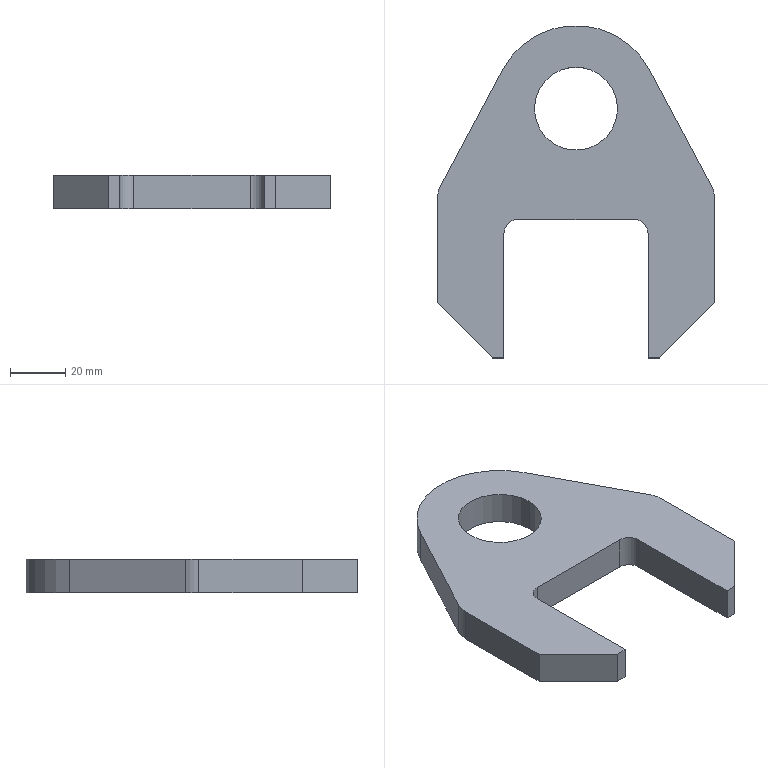Part | SolidWorks | features Extrusion 1 | 1 solid | 20 faces | box 100 x 120 x 12 mm | volume 75307 mm3 | plane 13 | cylinder 7 | commonest cylinder face diameters 10 x2 20 x2 30 x2 60 x1
STEP:
#1=CARTESIAN_POINT('',(-15.,90.,6.));
#2=VERTEX_POINT('',#1);
#3=CARTESIAN_POINT('',(15.,90.,6.));
#4=VERTEX_POINT('',#3);
#5=CARTESIAN_POINT('',(0.,90.,6.));
#6=DIRECTION('',(0.,0.,1.));
#7=DIRECTION('',(1.,0.,0.));
#8=AXIS2_PLACEMENT_3D('',#5,#6,#7);
#9=CIRCLE('',#8,15.);
#10=EDGE_CURVE('',#2,#4,#9,.T.);
#11=ORIENTED_EDGE('',*,*,#10,.T.);
#12=CARTESIAN_POINT('',(15.,90.,-6.));
#13=VERTEX_POINT('',#12);
#14=CARTESIAN_POINT('',(15.,90.,6.));
#15=DIRECTION('',(0.,0.,-1.));
#16=VECTOR('',#15,1000.);
#17=LINE('',#14,#16);
#18=EDGE_CURVE('',#4,#13,#17,.T.);
#19=ORIENTED_EDGE('',*,*,#18,.T.);
#20=CARTESIAN_POINT('',(-15.,90.,-6.));
#21=VERTEX_POINT('',#20);
#22=CARTESIAN_POINT('',(0.,90.,-6.));
#23=DIRECTION('',(0.,0.,1.));
#24=DIRECTION('',(1.,0.,0.));
#25=AXIS2_PLACEMENT_3D('',#22,#23,#24);
#26=CIRCLE('',#25,15.);
#27=EDGE_CURVE('',#21,#13,#26,.T.);
#28=ORIENTED_EDGE('',*,*,#27,.F.);
#29=CARTESIAN_POINT('',(-15.,90.,6.));
#30=DIRECTION('',(0.,0.,-1.));
#31=VECTOR('',#30,1000.);
#32=LINE('',#29,#31);
#33=EDGE_CURVE('',#2,#21,#32,.T.);
#34=ORIENTED_EDGE('',*,*,#33,.F.);
#35=EDGE_LOOP('',(#11,#19,#28,#34));
#36=FACE_OUTER_BOUND('',#35,.T.);
#37=CARTESIAN_POINT('',(0.,90.,6.));
#38=DIRECTION('',(0.,0.,-1.));
#39=DIRECTION('',(-1.,0.,0.));
#40=AXIS2_PLACEMENT_3D('',#37,#38,#39);
#41=CYLINDRICAL_SURFACE('',#40,15.);
#42=ADVANCED_FACE('',(#36),#41,.F.);
#43=CARTESIAN_POINT('',(-26.,0.,6.));
#44=VERTEX_POINT('',#43);
#45=CARTESIAN_POINT('',(-26.,45.,6.));
#46=VERTEX_POINT('',#45);
#47=CARTESIAN_POINT('',(-26.,0.,6.));
#48=DIRECTION('',(0.,1.,0.));
#49=VECTOR('',#48,1000.);
#50=LINE('',#47,#49);
#51=EDGE_CURVE('',#44,#46,#50,.T.);
#52=ORIENTED_EDGE('',*,*,#51,.T.);
#53=CARTESIAN_POINT('',(-21.,50.,6.));
#54=VERTEX_POINT('',#53);
#55=CARTESIAN_POINT('',(-21.,45.,6.));
#56=DIRECTION('',(0.,0.,-1.));
#57=DIRECTION('',(-1.,0.,0.));
#58=AXIS2_PLACEMENT_3D('',#55,#56,#57);
#59=CIRCLE('',#58,5.);
#60=EDGE_CURVE('',#46,#54,#59,.T.);
#61=ORIENTED_EDGE('',*,*,#60,.T.);
#62=CARTESIAN_POINT('',(21.,50.,6.));
#63=VERTEX_POINT('',#62);
#64=CARTESIAN_POINT('',(-21.,50.,6.));
#65=DIRECTION('',(1.,0.,0.));
#66=VECTOR('',#65,1000.);
#67=LINE('',#64,#66);
#68=EDGE_CURVE('',#54,#63,#67,.T.);
#69=ORIENTED_EDGE('',*,*,#68,.T.);
#70=CARTESIAN_POINT('',(26.,45.,6.));
#71=VERTEX_POINT('',#70);
#72=CARTESIAN_POINT('',(21.,45.,6.));
#73=DIRECTION('',(0.,0.,-1.));
#74=DIRECTION('',(1.,0.,0.));
#75=AXIS2_PLACEMENT_3D('',#72,#73,#74);
#76=CIRCLE('',#75,5.);
#77=EDGE_CURVE('',#63,#71,#76,.T.);
#78=ORIENTED_EDGE('',*,*,#77,.T.);
#79=CARTESIAN_POINT('',(26.,0.,6.));
#80=VERTEX_POINT('',#79);
#81=CARTESIAN_POINT('',(26.,0.,6.));
#82=DIRECTION('',(0.,-1.,0.));
#83=VECTOR('',#82,1000.);
#84=LINE('',#81,#83);
#85=EDGE_CURVE('',#71,#80,#84,.T.);
#86=ORIENTED_EDGE('',*,*,#85,.T.);
#87=CARTESIAN_POINT('',(30.,0.,6.));
#88=VERTEX_POINT('',#87);
#89=CARTESIAN_POINT('',(26.,0.,6.));
#90=DIRECTION('',(1.,0.,0.));
#91=VECTOR('',#90,1000.);
#92=LINE('',#89,#91);
#93=EDGE_CURVE('',#80,#88,#92,.T.);
#94=ORIENTED_EDGE('',*,*,#93,.T.);
#95=CARTESIAN_POINT('',(50.,20.,6.));
#96=VERTEX_POINT('',#95);
#97=CARTESIAN_POINT('',(30.,0.,6.));
#98=DIRECTION('',(0.7071,0.7071,0.));
#99=VECTOR('',#98,1000.);
#100=LINE('',#97,#99);
#101=EDGE_CURVE('',#88,#96,#100,.T.);
#102=ORIENTED_EDGE('',*,*,#101,.T.);
#103=CARTESIAN_POINT('',(50.,57.5,6.));
#104=VERTEX_POINT('',#103);
#105=CARTESIAN_POINT('',(50.,20.,6.));
#106=DIRECTION('',(0.,1.,0.));
#107=VECTOR('',#106,1000.);
#108=LINE('',#105,#107);
#109=EDGE_CURVE('',#96,#104,#108,.T.);
#110=ORIENTED_EDGE('',*,*,#109,.T.);
#111=CARTESIAN_POINT('',(48.824,62.206,6.));
#112=VERTEX_POINT('',#111);
#113=CARTESIAN_POINT('',(40.,57.5,6.));
#114=DIRECTION('',(0.,0.,1.));
#115=DIRECTION('',(-1.,0.,0.));
#116=AXIS2_PLACEMENT_3D('',#113,#114,#115);
#117=CIRCLE('',#116,10.);
#118=EDGE_CURVE('',#104,#112,#117,.T.);
#119=ORIENTED_EDGE('',*,*,#118,.T.);
#120=CARTESIAN_POINT('',(26.471,104.118,6.));
#121=VERTEX_POINT('',#120);
#122=CARTESIAN_POINT('',(48.824,62.206,6.));
#123=DIRECTION('',(-0.4706,0.8824,0.));
#124=VECTOR('',#123,1000.);
#125=LINE('',#122,#124);
#126=EDGE_CURVE('',#112,#121,#125,.T.);
#127=ORIENTED_EDGE('',*,*,#126,.T.);
#128=CARTESIAN_POINT('',(-26.471,104.118,6.));
#129=VERTEX_POINT('',#128);
#130=CARTESIAN_POINT('',(0.,90.,6.));
#131=DIRECTION('',(0.,0.,1.));
#132=DIRECTION('',(-1.,0.,0.));
#133=AXIS2_PLACEMENT_3D('',#130,#131,#132);
#134=CIRCLE('',#133,30.);
#135=EDGE_CURVE('',#121,#129,#134,.T.);
#136=ORIENTED_EDGE('',*,*,#135,.T.);
#137=CARTESIAN_POINT('',(-48.824,62.206,6.));
#138=VERTEX_POINT('',#137);
#139=CARTESIAN_POINT('',(-48.824,62.206,6.));
#140=DIRECTION('',(-0.4706,-0.8824,0.));
#141=VECTOR('',#140,1000.);
#142=LINE('',#139,#141);
#143=EDGE_CURVE('',#129,#138,#142,.T.);
#144=ORIENTED_EDGE('',*,*,#143,.T.);
#145=CARTESIAN_POINT('',(-50.,57.5,6.));
#146=VERTEX_POINT('',#145);
#147=CARTESIAN_POINT('',(-40.,57.5,6.));
#148=DIRECTION('',(0.,0.,1.));
#149=DIRECTION('',(-1.,0.,0.));
#150=AXIS2_PLACEMENT_3D('',#147,#148,#149);
#151=CIRCLE('',#150,10.);
#152=EDGE_CURVE('',#138,#146,#151,.T.);
#153=ORIENTED_EDGE('',*,*,#152,.T.);
#154=CARTESIAN_POINT('',(-50.,20.,6.));
#155=VERTEX_POINT('',#154);
#156=CARTESIAN_POINT('',(-50.,20.,6.));
#157=DIRECTION('',(0.,-1.,0.));
#158=VECTOR('',#157,1000.);
#159=LINE('',#156,#158);
#160=EDGE_CURVE('',#146,#155,#159,.T.);
#161=ORIENTED_EDGE('',*,*,#160,.T.);
#162=CARTESIAN_POINT('',(-30.,0.,6.));
#163=VERTEX_POINT('',#162);
#164=CARTESIAN_POINT('',(-30.,0.,6.));
#165=DIRECTION('',(0.7071,-0.7071,0.));
#166=VECTOR('',#165,1000.);
#167=LINE('',#164,#166);
#168=EDGE_CURVE('',#155,#163,#167,.T.);
#169=ORIENTED_EDGE('',*,*,#168,.T.);
#170=CARTESIAN_POINT('',(-26.,0.,6.));
#171=DIRECTION('',(1.,0.,0.));
#172=VECTOR('',#171,1000.);
#173=LINE('',#170,#172);
#174=EDGE_CURVE('',#163,#44,#173,.T.);
#175=ORIENTED_EDGE('',*,*,#174,.T.);
#176=EDGE_LOOP('',(#52,#61,#69,#78,#86,#94,#102,#110,#119,#127,#136,#144,#153,#161,#169,#175));
#177=FACE_OUTER_BOUND('',#176,.T.);
#178=ORIENTED_EDGE('',*,*,#10,.F.);
#179=CARTESIAN_POINT('',(0.,90.,6.));
#180=DIRECTION('',(0.,0.,1.));
#181=DIRECTION('',(1.,0.,0.));
#182=AXIS2_PLACEMENT_3D('',#179,#180,#181);
#183=CIRCLE('',#182,15.);
#184=EDGE_CURVE('',#4,#2,#183,.T.);
#185=ORIENTED_EDGE('',*,*,#184,.F.);
#186=EDGE_LOOP('',(#178,#185));
#187=FACE_BOUND('',#186,.T.);
#188=CARTESIAN_POINT('',(-21.,45.,6.));
#189=DIRECTION('',(0.,0.,-1.));
#190=DIRECTION('',(-1.,0.,0.));
#191=AXIS2_PLACEMENT_3D('',#188,#189,#190);
#192=PLANE('',#191);
#193=ADVANCED_FACE('',(#177,#187),#192,.F.);
#194=CARTESIAN_POINT('',(-26.,0.,-6.));
#195=VERTEX_POINT('',#194);
#196=CARTESIAN_POINT('',(-26.,45.,-6.));
#197=VERTEX_POINT('',#196);
#198=CARTESIAN_POINT('',(-26.,0.,-6.));
#199=DIRECTION('',(0.,1.,0.));
#200=VECTOR('',#199,1000.);
#201=LINE('',#198,#200);
#202=EDGE_CURVE('',#195,#197,#201,.T.);
#203=ORIENTED_EDGE('',*,*,#202,.F.);
#204=CARTESIAN_POINT('',(-30.,0.,-6.));
#205=VERTEX_POINT('',#204);
#206=CARTESIAN_POINT('',(-26.,0.,-6.));
#207=DIRECTION('',(1.,0.,0.));
#208=VECTOR('',#207,1000.);
#209=LINE('',#206,#208);
#210=EDGE_CURVE('',#205,#195,#209,.T.);
#211=ORIENTED_EDGE('',*,*,#210,.F.);
#212=CARTESIAN_POINT('',(-50.,20.,-6.));
#213=VERTEX_POINT('',#212);
#214=CARTESIAN_POINT('',(-30.,0.,-6.));
#215=DIRECTION('',(0.7071,-0.7071,0.));
#216=VECTOR('',#215,1000.);
#217=LINE('',#214,#216);
#218=EDGE_CURVE('',#213,#205,#217,.T.);
#219=ORIENTED_EDGE('',*,*,#218,.F.);
#220=CARTESIAN_POINT('',(-50.,57.5,-6.));
#221=VERTEX_POINT('',#220);
#222=CARTESIAN_POINT('',(-50.,20.,-6.));
#223=DIRECTION('',(0.,-1.,0.));
#224=VECTOR('',#223,1000.);
#225=LINE('',#222,#224);
#226=EDGE_CURVE('',#221,#213,#225,.T.);
#227=ORIENTED_EDGE('',*,*,#226,.F.);
#228=CARTESIAN_POINT('',(-48.824,62.206,-6.));
#229=VERTEX_POINT('',#228);
#230=CARTESIAN_POINT('',(-40.,57.5,-6.));
#231=DIRECTION('',(0.,0.,1.));
#232=DIRECTION('',(-1.,0.,0.));
#233=AXIS2_PLACEMENT_3D('',#230,#231,#232);
#234=CIRCLE('',#233,10.);
#235=EDGE_CURVE('',#229,#221,#234,.T.);
#236=ORIENTED_EDGE('',*,*,#235,.F.);
#237=CARTESIAN_POINT('',(-26.471,104.118,-6.));
#238=VERTEX_POINT('',#237);
#239=CARTESIAN_POINT('',(-48.824,62.206,-6.));
#240=DIRECTION('',(-0.4706,-0.8824,0.));
#241=VECTOR('',#240,1000.);
#242=LINE('',#239,#241);
#243=EDGE_CURVE('',#238,#229,#242,.T.);
#244=ORIENTED_EDGE('',*,*,#243,.F.);
#245=CARTESIAN_POINT('',(26.471,104.118,-6.));
#246=VERTEX_POINT('',#245);
#247=CARTESIAN_POINT('',(0.,90.,-6.));
#248=DIRECTION('',(0.,0.,1.));
#249=DIRECTION('',(-1.,0.,0.));
#250=AXIS2_PLACEMENT_3D('',#247,#248,#249);
#251=CIRCLE('',#250,30.);
#252=EDGE_CURVE('',#246,#238,#251,.T.);
#253=ORIENTED_EDGE('',*,*,#252,.F.);
#254=CARTESIAN_POINT('',(48.824,62.206,-6.));
#255=VERTEX_POINT('',#254);
#256=CARTESIAN_POINT('',(48.824,62.206,-6.));
#257=DIRECTION('',(-0.4706,0.8824,0.));
#258=VECTOR('',#257,1000.);
#259=LINE('',#256,#258);
#260=EDGE_CURVE('',#255,#246,#259,.T.);
#261=ORIENTED_EDGE('',*,*,#260,.F.);
#262=CARTESIAN_POINT('',(50.,57.5,-6.));
#263=VERTEX_POINT('',#262);
#264=CARTESIAN_POINT('',(40.,57.5,-6.));
#265=DIRECTION('',(0.,0.,1.));
#266=DIRECTION('',(-1.,0.,0.));
#267=AXIS2_PLACEMENT_3D('',#264,#265,#266);
#268=CIRCLE('',#267,10.);
#269=EDGE_CURVE('',#263,#255,#268,.T.);
#270=ORIENTED_EDGE('',*,*,#269,.F.);
#271=CARTESIAN_POINT('',(50.,20.,-6.));
#272=VERTEX_POINT('',#271);
#273=CARTESIAN_POINT('',(50.,20.,-6.));
#274=DIRECTION('',(0.,1.,0.));
#275=VECTOR('',#274,1000.);
#276=LINE('',#273,#275);
#277=EDGE_CURVE('',#272,#263,#276,.T.);
#278=ORIENTED_EDGE('',*,*,#277,.F.);
#279=CARTESIAN_POINT('',(30.,0.,-6.));
#280=VERTEX_POINT('',#279);
#281=CARTESIAN_POINT('',(30.,0.,-6.));
#282=DIRECTION('',(0.7071,0.7071,0.));
#283=VECTOR('',#282,1000.);
#284=LINE('',#281,#283);
#285=EDGE_CURVE('',#280,#272,#284,.T.);
#286=ORIENTED_EDGE('',*,*,#285,.F.);
#287=CARTESIAN_POINT('',(26.,0.,-6.));
#288=VERTEX_POINT('',#287);
#289=CARTESIAN_POINT('',(26.,0.,-6.));
#290=DIRECTION('',(1.,0.,0.));
#291=VECTOR('',#290,1000.);
#292=LINE('',#289,#291);
#293=EDGE_CURVE('',#288,#280,#292,.T.);
#294=ORIENTED_EDGE('',*,*,#293,.F.);
#295=CARTESIAN_POINT('',(26.,45.,-6.));
#296=VERTEX_POINT('',#295);
#297=CARTESIAN_POINT('',(26.,0.,-6.));
#298=DIRECTION('',(0.,-1.,0.));
#299=VECTOR('',#298,1000.);
#300=LINE('',#297,#299);
#301=EDGE_CURVE('',#296,#288,#300,.T.);
#302=ORIENTED_EDGE('',*,*,#301,.F.);
#303=CARTESIAN_POINT('',(21.,50.,-6.));
#304=VERTEX_POINT('',#303);
#305=CARTESIAN_POINT('',(21.,45.,-6.));
#306=DIRECTION('',(0.,0.,-1.));
#307=DIRECTION('',(1.,0.,0.));
#308=AXIS2_PLACEMENT_3D('',#305,#306,#307);
#309=CIRCLE('',#308,5.);
#310=EDGE_CURVE('',#304,#296,#309,.T.);
#311=ORIENTED_EDGE('',*,*,#310,.F.);
#312=CARTESIAN_POINT('',(-21.,50.,-6.));
#313=VERTEX_POINT('',#312);
#314=CARTESIAN_POINT('',(-21.,50.,-6.));
#315=DIRECTION('',(1.,0.,0.));
#316=VECTOR('',#315,1000.);
#317=LINE('',#314,#316);
#318=EDGE_CURVE('',#313,#304,#317,.T.);
#319=ORIENTED_EDGE('',*,*,#318,.F.);
#320=CARTESIAN_POINT('',(-21.,45.,-6.));
#321=DIRECTION('',(0.,0.,-1.));
#322=DIRECTION('',(-1.,0.,0.));
#323=AXIS2_PLACEMENT_3D('',#320,#321,#322);
#324=CIRCLE('',#323,5.);
#325=EDGE_CURVE('',#197,#313,#324,.T.);
#326=ORIENTED_EDGE('',*,*,#325,.F.);
#327=EDGE_LOOP('',(#203,#211,#219,#227,#236,#244,#253,#261,#270,#278,#286,#294,#302,#311,#319,#326));
#328=FACE_OUTER_BOUND('',#327,.T.);
#329=ORIENTED_EDGE('',*,*,#27,.T.);
#330=CARTESIAN_POINT('',(0.,90.,-6.));
#331=DIRECTION('',(0.,0.,1.));
#332=DIRECTION('',(1.,0.,0.));
#333=AXIS2_PLACEMENT_3D('',#330,#331,#332);
#334=CIRCLE('',#333,15.);
#335=EDGE_CURVE('',#13,#21,#334,.T.);
#336=ORIENTED_EDGE('',*,*,#335,.T.);
#337=EDGE_LOOP('',(#329,#336));
#338=FACE_BOUND('',#337,.T.);
#339=CARTESIAN_POINT('',(-21.,45.,-6.));
#340=DIRECTION('',(0.,0.,-1.));
#341=DIRECTION('',(-1.,0.,0.));
#342=AXIS2_PLACEMENT_3D('',#339,#340,#341);
#343=PLANE('',#342);
#344=ADVANCED_FACE('',(#328,#338),#343,.T.);
#345=ORIENTED_EDGE('',*,*,#202,.T.);
#346=CARTESIAN_POINT('',(-26.,45.,6.));
#347=DIRECTION('',(0.,0.,-1.));
#348=VECTOR('',#347,1000.);
#349=LINE('',#346,#348);
#350=EDGE_CURVE('',#46,#197,#349,.T.);
#351=ORIENTED_EDGE('',*,*,#350,.F.);
#352=ORIENTED_EDGE('',*,*,#51,.F.);
#353=CARTESIAN_POINT('',(-26.,0.,6.));
#354=DIRECTION('',(0.,0.,-1.));
#355=VECTOR('',#354,1000.);
#356=LINE('',#353,#355);
#357=EDGE_CURVE('',#44,#195,#356,.T.);
#358=ORIENTED_EDGE('',*,*,#357,.T.);
#359=EDGE_LOOP('',(#345,#351,#352,#358));
#360=FACE_OUTER_BOUND('',#359,.T.);
#361=CARTESIAN_POINT('',(-26.,0.,6.));
#362=DIRECTION('',(-1.,0.,0.));
#363=DIRECTION('',(0.,0.,1.));
#364=AXIS2_PLACEMENT_3D('',#361,#362,#363);
#365=PLANE('',#364);
#366=ADVANCED_FACE('',(#360),#365,.F.);
#367=ORIENTED_EDGE('',*,*,#325,.T.);
#368=CARTESIAN_POINT('',(-21.,50.,6.));
#369=DIRECTION('',(0.,0.,-1.));
#370=VECTOR('',#369,1000.);
#371=LINE('',#368,#370);
#372=EDGE_CURVE('',#54,#313,#371,.T.);
#373=ORIENTED_EDGE('',*,*,#372,.F.);
#374=ORIENTED_EDGE('',*,*,#60,.F.);
#375=ORIENTED_EDGE('',*,*,#350,.T.);
#376=EDGE_LOOP('',(#367,#373,#374,#375));
#377=FACE_OUTER_BOUND('',#376,.T.);
#378=CARTESIAN_POINT('',(-21.,45.,6.));
#379=DIRECTION('',(0.,0.,-1.));
#380=DIRECTION('',(-1.,0.,0.));
#381=AXIS2_PLACEMENT_3D('',#378,#379,#380);
#382=CYLINDRICAL_SURFACE('',#381,5.);
#383=ADVANCED_FACE('',(#377),#382,.F.);
#384=ORIENTED_EDGE('',*,*,#318,.T.);
#385=CARTESIAN_POINT('',(21.,50.,6.));
#386=DIRECTION('',(0.,0.,-1.));
#387=VECTOR('',#386,1000.);
#388=LINE('',#385,#387);
#389=EDGE_CURVE('',#63,#304,#388,.T.);
#390=ORIENTED_EDGE('',*,*,#389,.F.);
#391=ORIENTED_EDGE('',*,*,#68,.F.);
#392=ORIENTED_EDGE('',*,*,#372,.T.);
#393=EDGE_LOOP('',(#384,#390,#391,#392));
#394=FACE_OUTER_BOUND('',#393,.T.);
#395=CARTESIAN_POINT('',(-21.,50.,6.));
#396=DIRECTION('',(0.,1.,0.));
#397=DIRECTION('',(0.,0.,1.));
#398=AXIS2_PLACEMENT_3D('',#395,#396,#397);
#399=PLANE('',#398);
#400=ADVANCED_FACE('',(#394),#399,.F.);
#401=ORIENTED_EDGE('',*,*,#310,.T.);
#402=CARTESIAN_POINT('',(26.,45.,6.));
#403=DIRECTION('',(0.,0.,-1.));
#404=VECTOR('',#403,1000.);
#405=LINE('',#402,#404);
#406=EDGE_CURVE('',#71,#296,#405,.T.);
#407=ORIENTED_EDGE('',*,*,#406,.F.);
#408=ORIENTED_EDGE('',*,*,#77,.F.);
#409=ORIENTED_EDGE('',*,*,#389,.T.);
#410=EDGE_LOOP('',(#401,#407,#408,#409));
#411=FACE_OUTER_BOUND('',#410,.T.);
#412=CARTESIAN_POINT('',(21.,45.,6.));
#413=DIRECTION('',(0.,0.,-1.));
#414=DIRECTION('',(-1.,0.,0.));
#415=AXIS2_PLACEMENT_3D('',#412,#413,#414);
#416=CYLINDRICAL_SURFACE('',#415,5.);
#417=ADVANCED_FACE('',(#411),#416,.F.);
#418=ORIENTED_EDGE('',*,*,#301,.T.);
#419=CARTESIAN_POINT('',(26.,0.,6.));
#420=DIRECTION('',(0.,0.,-1.));
#421=VECTOR('',#420,1000.);
#422=LINE('',#419,#421);
#423=EDGE_CURVE('',#80,#288,#422,.T.);
#424=ORIENTED_EDGE('',*,*,#423,.F.);
#425=ORIENTED_EDGE('',*,*,#85,.F.);
#426=ORIENTED_EDGE('',*,*,#406,.T.);
#427=EDGE_LOOP('',(#418,#424,#425,#426));
#428=FACE_OUTER_BOUND('',#427,.T.);
#429=CARTESIAN_POINT('',(26.,0.,6.));
#430=DIRECTION('',(1.,0.,0.));
#431=DIRECTION('',(0.,0.,-1.));
#432=AXIS2_PLACEMENT_3D('',#429,#430,#431);
#433=PLANE('',#432);
#434=ADVANCED_FACE('',(#428),#433,.F.);
#435=ORIENTED_EDGE('',*,*,#293,.T.);
#436=CARTESIAN_POINT('',(30.,0.,6.));
#437=DIRECTION('',(0.,0.,-1.));
#438=VECTOR('',#437,1000.);
#439=LINE('',#436,#438);
#440=EDGE_CURVE('',#88,#280,#439,.T.);
#441=ORIENTED_EDGE('',*,*,#440,.F.);
#442=ORIENTED_EDGE('',*,*,#93,.F.);
#443=ORIENTED_EDGE('',*,*,#423,.T.);
#444=EDGE_LOOP('',(#435,#441,#442,#443));
#445=FACE_OUTER_BOUND('',#444,.T.);
#446=CARTESIAN_POINT('',(26.,0.,6.));
#447=DIRECTION('',(0.,1.,0.));
#448=DIRECTION('',(-1.,0.,0.));
#449=AXIS2_PLACEMENT_3D('',#446,#447,#448);
#450=PLANE('',#449);
#451=ADVANCED_FACE('',(#445),#450,.F.);
#452=ORIENTED_EDGE('',*,*,#285,.T.);
#453=CARTESIAN_POINT('',(50.,20.,6.));
#454=DIRECTION('',(0.,0.,-1.));
#455=VECTOR('',#454,1000.);
#456=LINE('',#453,#455);
#457=EDGE_CURVE('',#96,#272,#456,.T.);
#458=ORIENTED_EDGE('',*,*,#457,.F.);
#459=ORIENTED_EDGE('',*,*,#101,.F.);
#460=ORIENTED_EDGE('',*,*,#440,.T.);
#461=EDGE_LOOP('',(#452,#458,#459,#460));
#462=FACE_OUTER_BOUND('',#461,.T.);
#463=CARTESIAN_POINT('',(30.,0.,6.));
#464=DIRECTION('',(-0.7071,0.7071,0.));
#465=DIRECTION('',(-0.7071,-0.7071,0.));
#466=AXIS2_PLACEMENT_3D('',#463,#464,#465);
#467=PLANE('',#466);
#468=ADVANCED_FACE('',(#462),#467,.F.);
#469=ORIENTED_EDGE('',*,*,#277,.T.);
#470=CARTESIAN_POINT('',(50.,57.5,6.));
#471=DIRECTION('',(0.,0.,-1.));
#472=VECTOR('',#471,1000.);
#473=LINE('',#470,#472);
#474=EDGE_CURVE('',#104,#263,#473,.T.);
#475=ORIENTED_EDGE('',*,*,#474,.F.);
#476=ORIENTED_EDGE('',*,*,#109,.F.);
#477=ORIENTED_EDGE('',*,*,#457,.T.);
#478=EDGE_LOOP('',(#469,#475,#476,#477));
#479=FACE_OUTER_BOUND('',#478,.T.);
#480=CARTESIAN_POINT('',(50.,20.,6.));
#481=DIRECTION('',(-1.,0.,0.));
#482=DIRECTION('',(0.,0.,1.));
#483=AXIS2_PLACEMENT_3D('',#480,#481,#482);
#484=PLANE('',#483);
#485=ADVANCED_FACE('',(#479),#484,.F.);
#486=ORIENTED_EDGE('',*,*,#269,.T.);
#487=CARTESIAN_POINT('',(48.824,62.206,6.));
#488=DIRECTION('',(0.,0.,-1.));
#489=VECTOR('',#488,1000.);
#490=LINE('',#487,#489);
#491=EDGE_CURVE('',#112,#255,#490,.T.);
#492=ORIENTED_EDGE('',*,*,#491,.F.);
#493=ORIENTED_EDGE('',*,*,#118,.F.);
#494=ORIENTED_EDGE('',*,*,#474,.T.);
#495=EDGE_LOOP('',(#486,#492,#493,#494));
#496=FACE_OUTER_BOUND('',#495,.T.);
#497=CARTESIAN_POINT('',(40.,57.5,6.));
#498=DIRECTION('',(0.,0.,-1.));
#499=DIRECTION('',(-1.,0.,0.));
#500=AXIS2_PLACEMENT_3D('',#497,#498,#499);
#501=CYLINDRICAL_SURFACE('',#500,10.);
#502=ADVANCED_FACE('',(#496),#501,.T.);
#503=ORIENTED_EDGE('',*,*,#260,.T.);
#504=CARTESIAN_POINT('',(26.471,104.118,6.));
#505=DIRECTION('',(0.,0.,-1.));
#506=VECTOR('',#505,1000.);
#507=LINE('',#504,#506);
#508=EDGE_CURVE('',#121,#246,#507,.T.);
#509=ORIENTED_EDGE('',*,*,#508,.F.);
#510=ORIENTED_EDGE('',*,*,#126,.F.);
#511=ORIENTED_EDGE('',*,*,#491,.T.);
#512=EDGE_LOOP('',(#503,#509,#510,#511));
#513=FACE_OUTER_BOUND('',#512,.T.);
#514=CARTESIAN_POINT('',(48.824,62.206,6.));
#515=DIRECTION('',(-0.8824,-0.4706,0.));
#516=DIRECTION('',(0.4706,-0.8824,0.));
#517=AXIS2_PLACEMENT_3D('',#514,#515,#516);
#518=PLANE('',#517);
#519=ADVANCED_FACE('',(#513),#518,.F.);
#520=ORIENTED_EDGE('',*,*,#252,.T.);
#521=CARTESIAN_POINT('',(-26.471,104.118,6.));
#522=DIRECTION('',(0.,0.,-1.));
#523=VECTOR('',#522,1000.);
#524=LINE('',#521,#523);
#525=EDGE_CURVE('',#129,#238,#524,.T.);
#526=ORIENTED_EDGE('',*,*,#525,.F.);
#527=ORIENTED_EDGE('',*,*,#135,.F.);
#528=ORIENTED_EDGE('',*,*,#508,.T.);
#529=EDGE_LOOP('',(#520,#526,#527,#528));
#530=FACE_OUTER_BOUND('',#529,.T.);
#531=CARTESIAN_POINT('',(0.,90.,6.));
#532=DIRECTION('',(0.,0.,-1.));
#533=DIRECTION('',(-1.,0.,0.));
#534=AXIS2_PLACEMENT_3D('',#531,#532,#533);
#535=CYLINDRICAL_SURFACE('',#534,30.);
#536=ADVANCED_FACE('',(#530),#535,.T.);
#537=ORIENTED_EDGE('',*,*,#243,.T.);
#538=CARTESIAN_POINT('',(-48.824,62.206,6.));
#539=DIRECTION('',(0.,0.,-1.));
#540=VECTOR('',#539,1000.);
#541=LINE('',#538,#540);
#542=EDGE_CURVE('',#138,#229,#541,.T.);
#543=ORIENTED_EDGE('',*,*,#542,.F.);
#544=ORIENTED_EDGE('',*,*,#143,.F.);
#545=ORIENTED_EDGE('',*,*,#525,.T.);
#546=EDGE_LOOP('',(#537,#543,#544,#545));
#547=FACE_OUTER_BOUND('',#546,.T.);
#548=CARTESIAN_POINT('',(-48.824,62.206,6.));
#549=DIRECTION('',(0.8824,-0.4706,0.));
#550=DIRECTION('',(0.4706,0.8824,0.));
#551=AXIS2_PLACEMENT_3D('',#548,#549,#550);
#552=PLANE('',#551);
#553=ADVANCED_FACE('',(#547),#552,.F.);
#554=ORIENTED_EDGE('',*,*,#235,.T.);
#555=CARTESIAN_POINT('',(-50.,57.5,6.));
#556=DIRECTION('',(0.,0.,-1.));
#557=VECTOR('',#556,1000.);
#558=LINE('',#555,#557);
#559=EDGE_CURVE('',#146,#221,#558,.T.);
#560=ORIENTED_EDGE('',*,*,#559,.F.);
#561=ORIENTED_EDGE('',*,*,#152,.F.);
#562=ORIENTED_EDGE('',*,*,#542,.T.);
#563=EDGE_LOOP('',(#554,#560,#561,#562));
#564=FACE_OUTER_BOUND('',#563,.T.);
#565=CARTESIAN_POINT('',(-40.,57.5,6.));
#566=DIRECTION('',(0.,0.,-1.));
#567=DIRECTION('',(-1.,0.,0.));
#568=AXIS2_PLACEMENT_3D('',#565,#566,#567);
#569=CYLINDRICAL_SURFACE('',#568,10.);
#570=ADVANCED_FACE('',(#564),#569,.T.);
#571=ORIENTED_EDGE('',*,*,#226,.T.);
#572=CARTESIAN_POINT('',(-50.,20.,6.));
#573=DIRECTION('',(0.,0.,-1.));
#574=VECTOR('',#573,1000.);
#575=LINE('',#572,#574);
#576=EDGE_CURVE('',#155,#213,#575,.T.);
#577=ORIENTED_EDGE('',*,*,#576,.F.);
#578=ORIENTED_EDGE('',*,*,#160,.F.);
#579=ORIENTED_EDGE('',*,*,#559,.T.);
#580=EDGE_LOOP('',(#571,#577,#578,#579));
#581=FACE_OUTER_BOUND('',#580,.T.);
#582=CARTESIAN_POINT('',(-50.,20.,6.));
#583=DIRECTION('',(1.,0.,0.));
#584=DIRECTION('',(0.,0.,-1.));
#585=AXIS2_PLACEMENT_3D('',#582,#583,#584);
#586=PLANE('',#585);
#587=ADVANCED_FACE('',(#581),#586,.F.);
#588=ORIENTED_EDGE('',*,*,#218,.T.);
#589=CARTESIAN_POINT('',(-30.,0.,6.));
#590=DIRECTION('',(0.,0.,-1.));
#591=VECTOR('',#590,1000.);
#592=LINE('',#589,#591);
#593=EDGE_CURVE('',#163,#205,#592,.T.);
#594=ORIENTED_EDGE('',*,*,#593,.F.);
#595=ORIENTED_EDGE('',*,*,#168,.F.);
#596=ORIENTED_EDGE('',*,*,#576,.T.);
#597=EDGE_LOOP('',(#588,#594,#595,#596));
#598=FACE_OUTER_BOUND('',#597,.T.);
#599=CARTESIAN_POINT('',(-30.,0.,6.));
#600=DIRECTION('',(0.7071,0.7071,0.));
#601=DIRECTION('',(-0.7071,0.7071,0.));
#602=AXIS2_PLACEMENT_3D('',#599,#600,#601);
#603=PLANE('',#602);
#604=ADVANCED_FACE('',(#598),#603,.F.);
#605=ORIENTED_EDGE('',*,*,#210,.T.);
#606=ORIENTED_EDGE('',*,*,#357,.F.);
#607=ORIENTED_EDGE('',*,*,#174,.F.);
#608=ORIENTED_EDGE('',*,*,#593,.T.);
#609=EDGE_LOOP('',(#605,#606,#607,#608));
#610=FACE_OUTER_BOUND('',#609,.T.);
#611=CARTESIAN_POINT('',(-26.,0.,6.));
#612=DIRECTION('',(0.,1.,0.));
#613=DIRECTION('',(-1.,0.,0.));
#614=AXIS2_PLACEMENT_3D('',#611,#612,#613);
#615=PLANE('',#614);
#616=ADVANCED_FACE('',(#610),#615,.F.);
#617=ORIENTED_EDGE('',*,*,#18,.F.);
#618=ORIENTED_EDGE('',*,*,#184,.T.);
#619=ORIENTED_EDGE('',*,*,#33,.T.);
#620=ORIENTED_EDGE('',*,*,#335,.F.);
#621=EDGE_LOOP('',(#617,#618,#619,#620));
#622=FACE_OUTER_BOUND('',#621,.T.);
#623=CARTESIAN_POINT('',(0.,90.,6.));
#624=DIRECTION('',(0.,0.,-1.));
#625=DIRECTION('',(-1.,0.,0.));
#626=AXIS2_PLACEMENT_3D('',#623,#624,#625);
#627=CYLINDRICAL_SURFACE('',#626,15.);
#628=ADVANCED_FACE('',(#622),#627,.F.);
#629=CLOSED_SHELL('',(#42,#193,#344,#366,#383,#400,#417,#434,#451,#468,#485,#502,#519,#536,#553,#570,#587,#604,#616,#628));
#630=MANIFOLD_SOLID_BREP('',#629);
#631=CARTESIAN_POINT('',(0.,0.,0.));
#632=DIRECTION('',(0.,0.,1.));
#633=DIRECTION('',(1.,0.,0.));
#634=AXIS2_PLACEMENT_3D('',#631,#632,#633);
#635=(LENGTH_UNIT()NAMED_UNIT(*)SI_UNIT(.MILLI.,.METRE.));
#636=UNCERTAINTY_MEASURE_WITH_UNIT(LENGTH_MEASURE(0.00001),#635,'','');
#637=(NAMED_UNIT(*)PLANE_ANGLE_UNIT()SI_UNIT($,.RADIAN.));
#638=(NAMED_UNIT(*)SI_UNIT($,.STERADIAN.)SOLID_ANGLE_UNIT());
#639=(GEOMETRIC_REPRESENTATION_CONTEXT(3)GLOBAL_UNCERTAINTY_ASSIGNED_CONTEXT((#636))GLOBAL_UNIT_ASSIGNED_CONTEXT((#635,#637,#638))REPRESENTATION_CONTEXT('',''));
#640=ADVANCED_BREP_SHAPE_REPRESENTATION('',(#630,#634),#639);